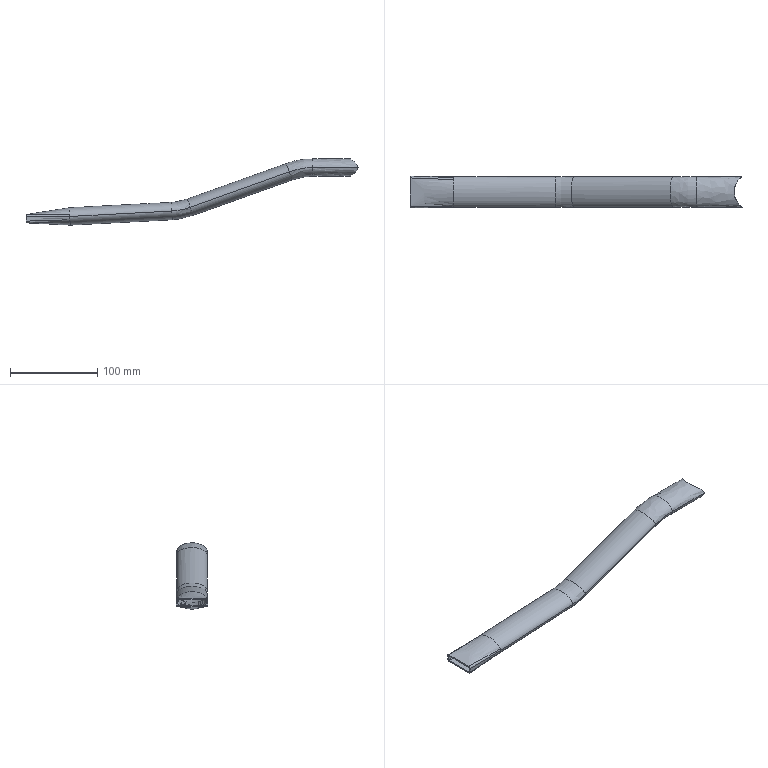Part | STEP file | PRT0001_68_11 | 1 solid | 55 faces | box 380.555 x 36.2 x 75.962 mm | volume 44196 mm3 | spline 32 | other 20 | plane 2 | cylinder 1 | commonest cylinder face diameters 43 x1